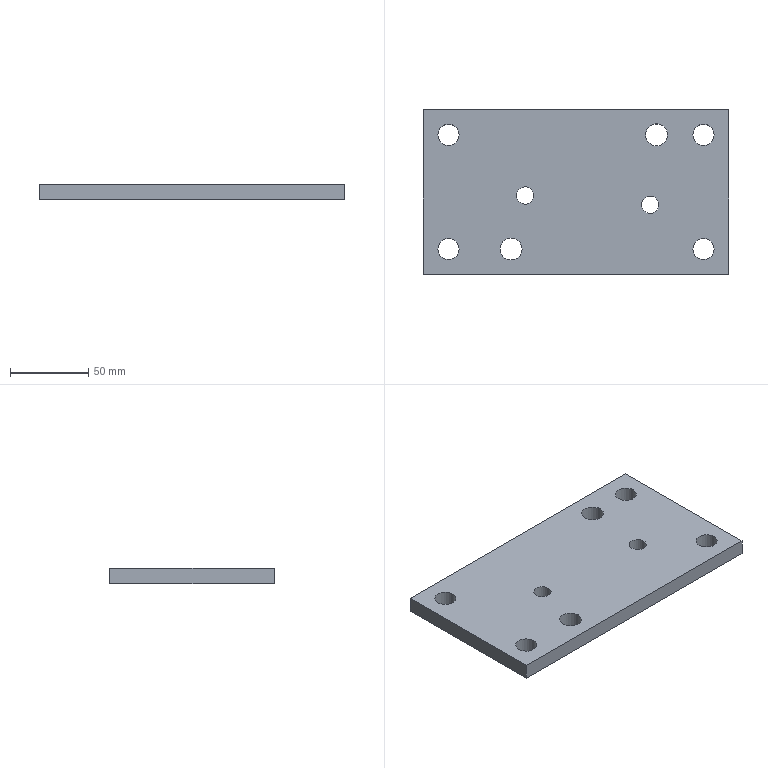Part | STEP file | lll_id2970_x_t | 1 solid | 14 faces | box 195 x 105 x 10 mm | volume 194037 mm3 | cylinder 8 | plane 6 | commonest cylinder face diameters 13.509 x4 11 x2 14 x2
STEP:
#1=CARTESIAN_POINT('',(1360.5,27.75,102.5));
#2=VERTEX_POINT('',#1);
#3=CARTESIAN_POINT('',(1366.,27.75,102.5));
#4=DIRECTION('',(0.,0.,-1.));
#5=DIRECTION('',(-1.,0.,0.));
#6=AXIS2_PLACEMENT_3D('',#3,#4,#5);
#7=CIRCLE('',#6,5.5);
#8=EDGE_CURVE('',#2,#2,#7,.T.);
#9=ORIENTED_EDGE('',*,*,#8,.F.);
#10=EDGE_LOOP('',(#9));
#11=FACE_BOUND('',#10,.T.);
#12=CARTESIAN_POINT('',(1360.5,27.75,92.5));
#13=VERTEX_POINT('',#12);
#14=CARTESIAN_POINT('',(1366.,27.75,92.5));
#15=DIRECTION('',(0.,0.,1.));
#16=DIRECTION('',(-1.,0.,0.));
#17=AXIS2_PLACEMENT_3D('',#14,#15,#16);
#18=CIRCLE('',#17,5.5);
#19=EDGE_CURVE('',#13,#13,#18,.T.);
#20=ORIENTED_EDGE('',*,*,#19,.F.);
#21=EDGE_LOOP('',(#20));
#22=FACE_BOUND('',#21,.T.);
#23=CARTESIAN_POINT('',(1366.,27.75,217.5));
#24=DIRECTION('',(0.,0.,-1.));
#25=DIRECTION('',(-1.,0.,0.));
#26=AXIS2_PLACEMENT_3D('',#23,#24,#25);
#27=CYLINDRICAL_SURFACE('',#26,5.5);
#28=ADVANCED_FACE('',(#11,#22),#27,.F.);
#29=CARTESIAN_POINT('',(1443.,66.5,102.5));
#30=VERTEX_POINT('',#29);
#31=CARTESIAN_POINT('',(1450.,66.5,102.5));
#32=DIRECTION('',(0.,0.,1.));
#33=DIRECTION('',(-1.,0.,0.));
#34=AXIS2_PLACEMENT_3D('',#31,#32,#33);
#35=CIRCLE('',#34,7.);
#36=EDGE_CURVE('',#30,#30,#35,.T.);
#37=ORIENTED_EDGE('',*,*,#36,.T.);
#38=EDGE_LOOP('',(#37));
#39=FACE_BOUND('',#38,.T.);
#40=CARTESIAN_POINT('',(1443.,66.5,92.5));
#41=VERTEX_POINT('',#40);
#42=CARTESIAN_POINT('',(1450.,66.5,92.5));
#43=DIRECTION('',(0.,0.,1.));
#44=DIRECTION('',(-1.,0.,0.));
#45=AXIS2_PLACEMENT_3D('',#42,#43,#44);
#46=CIRCLE('',#45,7.);
#47=EDGE_CURVE('',#41,#41,#46,.T.);
#48=ORIENTED_EDGE('',*,*,#47,.F.);
#49=EDGE_LOOP('',(#48));
#50=FACE_BOUND('',#49,.T.);
#51=CARTESIAN_POINT('',(1450.,66.5,92.5));
#52=DIRECTION('',(0.,0.,1.));
#53=DIRECTION('',(-1.,0.,0.));
#54=AXIS2_PLACEMENT_3D('',#51,#52,#53);
#55=CYLINDRICAL_SURFACE('',#54,7.);
#56=ADVANCED_FACE('',(#39,#50),#55,.F.);
#57=CARTESIAN_POINT('',(1310.245,66.5,102.5));
#58=VERTEX_POINT('',#57);
#59=CARTESIAN_POINT('',(1317.,66.5,102.5));
#60=DIRECTION('',(0.,0.,-1.));
#61=DIRECTION('',(-1.,0.,0.));
#62=AXIS2_PLACEMENT_3D('',#59,#60,#61);
#63=CIRCLE('',#62,6.755);
#64=EDGE_CURVE('',#58,#58,#63,.T.);
#65=ORIENTED_EDGE('',*,*,#64,.F.);
#66=EDGE_LOOP('',(#65));
#67=FACE_BOUND('',#66,.T.);
#68=CARTESIAN_POINT('',(1310.245,66.5,92.5));
#69=VERTEX_POINT('',#68);
#70=CARTESIAN_POINT('',(1317.,66.5,92.5));
#71=DIRECTION('',(0.,0.,1.));
#72=DIRECTION('',(-1.,0.,0.));
#73=AXIS2_PLACEMENT_3D('',#70,#71,#72);
#74=CIRCLE('',#73,6.755);
#75=EDGE_CURVE('',#69,#69,#74,.T.);
#76=ORIENTED_EDGE('',*,*,#75,.F.);
#77=EDGE_LOOP('',(#76));
#78=FACE_BOUND('',#77,.T.);
#79=CARTESIAN_POINT('',(1317.,66.5,92.5));
#80=DIRECTION('',(0.,0.,1.));
#81=DIRECTION('',(-1.,0.,0.));
#82=AXIS2_PLACEMENT_3D('',#79,#80,#81);
#83=CYLINDRICAL_SURFACE('',#82,6.755);
#84=ADVANCED_FACE('',(#67,#78),#83,.F.);
#85=CARTESIAN_POINT('',(1473.245,66.5,102.5));
#86=VERTEX_POINT('',#85);
#87=CARTESIAN_POINT('',(1480.,66.5,102.5));
#88=DIRECTION('',(0.,0.,-1.));
#89=DIRECTION('',(-1.,0.,0.));
#90=AXIS2_PLACEMENT_3D('',#87,#88,#89);
#91=CIRCLE('',#90,6.755);
#92=EDGE_CURVE('',#86,#86,#91,.T.);
#93=ORIENTED_EDGE('',*,*,#92,.F.);
#94=EDGE_LOOP('',(#93));
#95=FACE_BOUND('',#94,.T.);
#96=CARTESIAN_POINT('',(1473.245,66.5,92.5));
#97=VERTEX_POINT('',#96);
#98=CARTESIAN_POINT('',(1480.,66.5,92.5));
#99=DIRECTION('',(0.,0.,1.));
#100=DIRECTION('',(-1.,0.,0.));
#101=AXIS2_PLACEMENT_3D('',#98,#99,#100);
#102=CIRCLE('',#101,6.755);
#103=EDGE_CURVE('',#97,#97,#102,.T.);
#104=ORIENTED_EDGE('',*,*,#103,.F.);
#105=EDGE_LOOP('',(#104));
#106=FACE_BOUND('',#105,.T.);
#107=CARTESIAN_POINT('',(1480.,66.5,92.5));
#108=DIRECTION('',(0.,0.,1.));
#109=DIRECTION('',(-1.,0.,0.));
#110=AXIS2_PLACEMENT_3D('',#107,#108,#109);
#111=CYLINDRICAL_SURFACE('',#110,6.755);
#112=ADVANCED_FACE('',(#95,#106),#111,.F.);
#113=CARTESIAN_POINT('',(1301.,82.5,102.5));
#114=VERTEX_POINT('',#113);
#115=CARTESIAN_POINT('',(1301.,-22.5,102.5));
#116=VERTEX_POINT('',#115);
#117=CARTESIAN_POINT('',(1301.,30.,102.5));
#118=DIRECTION('',(0.,-1.,0.));
#119=VECTOR('',#118,1.);
#120=LINE('',#117,#119);
#121=EDGE_CURVE('',#114,#116,#120,.T.);
#122=ORIENTED_EDGE('',*,*,#121,.F.);
#123=CARTESIAN_POINT('',(1301.,82.5,92.5));
#124=VERTEX_POINT('',#123);
#125=CARTESIAN_POINT('',(1301.,82.5,92.5));
#126=DIRECTION('',(0.,0.,1.));
#127=VECTOR('',#126,1.);
#128=LINE('',#125,#127);
#129=EDGE_CURVE('',#124,#114,#128,.T.);
#130=ORIENTED_EDGE('',*,*,#129,.F.);
#131=CARTESIAN_POINT('',(1301.,-22.5,92.5));
#132=VERTEX_POINT('',#131);
#133=CARTESIAN_POINT('',(1301.,30.,92.5));
#134=DIRECTION('',(0.,-1.,0.));
#135=VECTOR('',#134,1.);
#136=LINE('',#133,#135);
#137=EDGE_CURVE('',#124,#132,#136,.T.);
#138=ORIENTED_EDGE('',*,*,#137,.T.);
#139=CARTESIAN_POINT('',(1301.,-22.5,92.5));
#140=DIRECTION('',(0.,0.,1.));
#141=VECTOR('',#140,1.);
#142=LINE('',#139,#141);
#143=EDGE_CURVE('',#132,#116,#142,.T.);
#144=ORIENTED_EDGE('',*,*,#143,.T.);
#145=EDGE_LOOP('',(#122,#130,#138,#144));
#146=FACE_OUTER_BOUND('',#145,.T.);
#147=CARTESIAN_POINT('',(1301.,30.,92.5));
#148=DIRECTION('',(-1.,0.,0.));
#149=DIRECTION('',(0.,0.,-1.));
#150=AXIS2_PLACEMENT_3D('',#147,#148,#149);
#151=PLANE('',#150);
#152=ADVANCED_FACE('',(#146),#151,.T.);
#153=CARTESIAN_POINT('',(1496.,-22.5,102.5));
#154=VERTEX_POINT('',#153);
#155=CARTESIAN_POINT('',(1398.5,-22.5,102.5));
#156=DIRECTION('',(-1.,0.,0.));
#157=VECTOR('',#156,1.);
#158=LINE('',#155,#157);
#159=EDGE_CURVE('',#154,#116,#158,.T.);
#160=ORIENTED_EDGE('',*,*,#159,.T.);
#161=ORIENTED_EDGE('',*,*,#143,.F.);
#162=CARTESIAN_POINT('',(1496.,-22.5,92.5));
#163=VERTEX_POINT('',#162);
#164=CARTESIAN_POINT('',(1398.5,-22.5,92.5));
#165=DIRECTION('',(1.,0.,0.));
#166=VECTOR('',#165,1.);
#167=LINE('',#164,#166);
#168=EDGE_CURVE('',#132,#163,#167,.T.);
#169=ORIENTED_EDGE('',*,*,#168,.T.);
#170=CARTESIAN_POINT('',(1496.,-22.5,92.5));
#171=DIRECTION('',(0.,0.,1.));
#172=VECTOR('',#171,1.);
#173=LINE('',#170,#172);
#174=EDGE_CURVE('',#163,#154,#173,.T.);
#175=ORIENTED_EDGE('',*,*,#174,.T.);
#176=EDGE_LOOP('',(#160,#161,#169,#175));
#177=FACE_OUTER_BOUND('',#176,.T.);
#178=CARTESIAN_POINT('',(1398.5,-22.5,92.5));
#179=DIRECTION('',(0.,-1.,0.));
#180=DIRECTION('',(0.,0.,1.));
#181=AXIS2_PLACEMENT_3D('',#178,#179,#180);
#182=PLANE('',#181);
#183=ADVANCED_FACE('',(#177),#182,.T.);
#184=CARTESIAN_POINT('',(1496.,82.5,102.5));
#185=VERTEX_POINT('',#184);
#186=CARTESIAN_POINT('',(1496.,30.,102.5));
#187=DIRECTION('',(0.,1.,0.));
#188=VECTOR('',#187,1.);
#189=LINE('',#186,#188);
#190=EDGE_CURVE('',#154,#185,#189,.T.);
#191=ORIENTED_EDGE('',*,*,#190,.F.);
#192=ORIENTED_EDGE('',*,*,#174,.F.);
#193=CARTESIAN_POINT('',(1496.,82.5,92.5));
#194=VERTEX_POINT('',#193);
#195=CARTESIAN_POINT('',(1496.,30.,92.5));
#196=DIRECTION('',(0.,1.,0.));
#197=VECTOR('',#196,1.);
#198=LINE('',#195,#197);
#199=EDGE_CURVE('',#163,#194,#198,.T.);
#200=ORIENTED_EDGE('',*,*,#199,.T.);
#201=CARTESIAN_POINT('',(1496.,82.5,92.5));
#202=DIRECTION('',(0.,0.,1.));
#203=VECTOR('',#202,1.);
#204=LINE('',#201,#203);
#205=EDGE_CURVE('',#194,#185,#204,.T.);
#206=ORIENTED_EDGE('',*,*,#205,.T.);
#207=EDGE_LOOP('',(#191,#192,#200,#206));
#208=FACE_OUTER_BOUND('',#207,.T.);
#209=CARTESIAN_POINT('',(1496.,30.,92.5));
#210=DIRECTION('',(1.,0.,0.));
#211=DIRECTION('',(0.,0.,1.));
#212=AXIS2_PLACEMENT_3D('',#209,#210,#211);
#213=PLANE('',#212);
#214=ADVANCED_FACE('',(#208),#213,.T.);
#215=CARTESIAN_POINT('',(1398.5,82.5,102.5));
#216=DIRECTION('',(1.,0.,0.));
#217=VECTOR('',#216,1.);
#218=LINE('',#215,#217);
#219=EDGE_CURVE('',#114,#185,#218,.T.);
#220=ORIENTED_EDGE('',*,*,#219,.T.);
#221=ORIENTED_EDGE('',*,*,#205,.F.);
#222=CARTESIAN_POINT('',(1398.5,82.5,92.5));
#223=DIRECTION('',(-1.,0.,0.));
#224=VECTOR('',#223,1.);
#225=LINE('',#222,#224);
#226=EDGE_CURVE('',#194,#124,#225,.T.);
#227=ORIENTED_EDGE('',*,*,#226,.T.);
#228=ORIENTED_EDGE('',*,*,#129,.T.);
#229=EDGE_LOOP('',(#220,#221,#227,#228));
#230=FACE_OUTER_BOUND('',#229,.T.);
#231=CARTESIAN_POINT('',(1398.5,82.5,92.5));
#232=DIRECTION('',(0.,1.,0.));
#233=DIRECTION('',(0.,0.,-1.));
#234=AXIS2_PLACEMENT_3D('',#231,#232,#233);
#235=PLANE('',#234);
#236=ADVANCED_FACE('',(#230),#235,.T.);
#237=CARTESIAN_POINT('',(1310.245,-6.5,102.5));
#238=VERTEX_POINT('',#237);
#239=CARTESIAN_POINT('',(1317.,-6.5,102.5));
#240=DIRECTION('',(0.,0.,-1.));
#241=DIRECTION('',(-1.,0.,0.));
#242=AXIS2_PLACEMENT_3D('',#239,#240,#241);
#243=CIRCLE('',#242,6.755);
#244=EDGE_CURVE('',#238,#238,#243,.T.);
#245=ORIENTED_EDGE('',*,*,#244,.F.);
#246=EDGE_LOOP('',(#245));
#247=FACE_BOUND('',#246,.T.);
#248=CARTESIAN_POINT('',(1310.245,-6.5,92.5));
#249=VERTEX_POINT('',#248);
#250=CARTESIAN_POINT('',(1317.,-6.5,92.5));
#251=DIRECTION('',(0.,0.,1.));
#252=DIRECTION('',(-1.,0.,0.));
#253=AXIS2_PLACEMENT_3D('',#250,#251,#252);
#254=CIRCLE('',#253,6.755);
#255=EDGE_CURVE('',#249,#249,#254,.T.);
#256=ORIENTED_EDGE('',*,*,#255,.F.);
#257=EDGE_LOOP('',(#256));
#258=FACE_BOUND('',#257,.T.);
#259=CARTESIAN_POINT('',(1317.,-6.5,92.5));
#260=DIRECTION('',(0.,0.,1.));
#261=DIRECTION('',(-1.,0.,0.));
#262=AXIS2_PLACEMENT_3D('',#259,#260,#261);
#263=CYLINDRICAL_SURFACE('',#262,6.755);
#264=ADVANCED_FACE('',(#247,#258),#263,.F.);
#265=CARTESIAN_POINT('',(1473.245,-6.5,102.5));
#266=VERTEX_POINT('',#265);
#267=CARTESIAN_POINT('',(1480.,-6.5,102.5));
#268=DIRECTION('',(0.,0.,1.));
#269=DIRECTION('',(-1.,0.,0.));
#270=AXIS2_PLACEMENT_3D('',#267,#268,#269);
#271=CIRCLE('',#270,6.755);
#272=EDGE_CURVE('',#266,#266,#271,.T.);
#273=ORIENTED_EDGE('',*,*,#272,.T.);
#274=EDGE_LOOP('',(#273));
#275=FACE_BOUND('',#274,.T.);
#276=CARTESIAN_POINT('',(1473.245,-6.5,92.5));
#277=VERTEX_POINT('',#276);
#278=CARTESIAN_POINT('',(1480.,-6.5,92.5));
#279=DIRECTION('',(0.,0.,1.));
#280=DIRECTION('',(-1.,0.,0.));
#281=AXIS2_PLACEMENT_3D('',#278,#279,#280);
#282=CIRCLE('',#281,6.755);
#283=EDGE_CURVE('',#277,#277,#282,.T.);
#284=ORIENTED_EDGE('',*,*,#283,.F.);
#285=EDGE_LOOP('',(#284));
#286=FACE_BOUND('',#285,.T.);
#287=CARTESIAN_POINT('',(1480.,-6.5,92.5));
#288=DIRECTION('',(0.,0.,1.));
#289=DIRECTION('',(-1.,0.,0.));
#290=AXIS2_PLACEMENT_3D('',#287,#288,#289);
#291=CYLINDRICAL_SURFACE('',#290,6.755);
#292=ADVANCED_FACE('',(#275,#286),#291,.F.);
#293=CARTESIAN_POINT('',(1350.,-6.5,102.5));
#294=VERTEX_POINT('',#293);
#295=CARTESIAN_POINT('',(1357.,-6.5,102.5));
#296=DIRECTION('',(0.,0.,1.));
#297=DIRECTION('',(-1.,0.,0.));
#298=AXIS2_PLACEMENT_3D('',#295,#296,#297);
#299=CIRCLE('',#298,7.);
#300=EDGE_CURVE('',#294,#294,#299,.T.);
#301=ORIENTED_EDGE('',*,*,#300,.T.);
#302=EDGE_LOOP('',(#301));
#303=FACE_BOUND('',#302,.T.);
#304=CARTESIAN_POINT('',(1350.,-6.5,92.5));
#305=VERTEX_POINT('',#304);
#306=CARTESIAN_POINT('',(1357.,-6.5,92.5));
#307=DIRECTION('',(0.,0.,1.));
#308=DIRECTION('',(-1.,0.,0.));
#309=AXIS2_PLACEMENT_3D('',#306,#307,#308);
#310=CIRCLE('',#309,7.);
#311=EDGE_CURVE('',#305,#305,#310,.T.);
#312=ORIENTED_EDGE('',*,*,#311,.F.);
#313=EDGE_LOOP('',(#312));
#314=FACE_BOUND('',#313,.T.);
#315=CARTESIAN_POINT('',(1357.,-6.5,92.5));
#316=DIRECTION('',(0.,0.,1.));
#317=DIRECTION('',(-1.,0.,0.));
#318=AXIS2_PLACEMENT_3D('',#315,#316,#317);
#319=CYLINDRICAL_SURFACE('',#318,7.);
#320=ADVANCED_FACE('',(#303,#314),#319,.F.);
#321=CARTESIAN_POINT('',(1440.5,21.75,92.5));
#322=VERTEX_POINT('',#321);
#323=CARTESIAN_POINT('',(1446.,21.75,92.5));
#324=DIRECTION('',(0.,0.,-1.));
#325=DIRECTION('',(-1.,0.,0.));
#326=AXIS2_PLACEMENT_3D('',#323,#324,#325);
#327=CIRCLE('',#326,5.5);
#328=EDGE_CURVE('',#322,#322,#327,.T.);
#329=ORIENTED_EDGE('',*,*,#328,.F.);
#330=EDGE_LOOP('',(#329));
#331=FACE_BOUND('',#330,.T.);
#332=ORIENTED_EDGE('',*,*,#311,.T.);
#333=EDGE_LOOP('',(#332));
#334=FACE_BOUND('',#333,.T.);
#335=ORIENTED_EDGE('',*,*,#283,.T.);
#336=EDGE_LOOP('',(#335));
#337=FACE_BOUND('',#336,.T.);
#338=ORIENTED_EDGE('',*,*,#255,.T.);
#339=EDGE_LOOP('',(#338));
#340=FACE_BOUND('',#339,.T.);
#341=ORIENTED_EDGE('',*,*,#137,.F.);
#342=ORIENTED_EDGE('',*,*,#226,.F.);
#343=ORIENTED_EDGE('',*,*,#199,.F.);
#344=ORIENTED_EDGE('',*,*,#168,.F.);
#345=EDGE_LOOP('',(#341,#342,#343,#344));
#346=FACE_BOUND('',#345,.T.);
#347=ORIENTED_EDGE('',*,*,#103,.T.);
#348=EDGE_LOOP('',(#347));
#349=FACE_BOUND('',#348,.T.);
#350=ORIENTED_EDGE('',*,*,#75,.T.);
#351=EDGE_LOOP('',(#350));
#352=FACE_BOUND('',#351,.T.);
#353=ORIENTED_EDGE('',*,*,#47,.T.);
#354=EDGE_LOOP('',(#353));
#355=FACE_BOUND('',#354,.T.);
#356=ORIENTED_EDGE('',*,*,#19,.T.);
#357=EDGE_LOOP('',(#356));
#358=FACE_BOUND('',#357,.T.);
#359=CARTESIAN_POINT('',(1398.5,30.,92.5));
#360=DIRECTION('',(0.,0.,-1.));
#361=DIRECTION('',(1.,0.,0.));
#362=AXIS2_PLACEMENT_3D('',#359,#360,#361);
#363=PLANE('',#362);
#364=ADVANCED_FACE('',(#331,#334,#337,#340,#346,#349,#352,#355,#358),#363,.T.);
#365=CARTESIAN_POINT('',(1440.5,21.75,102.5));
#366=VERTEX_POINT('',#365);
#367=CARTESIAN_POINT('',(1446.,21.75,102.5));
#368=DIRECTION('',(0.,0.,1.));
#369=DIRECTION('',(-1.,0.,0.));
#370=AXIS2_PLACEMENT_3D('',#367,#368,#369);
#371=CIRCLE('',#370,5.5);
#372=EDGE_CURVE('',#366,#366,#371,.T.);
#373=ORIENTED_EDGE('',*,*,#372,.T.);
#374=EDGE_LOOP('',(#373));
#375=FACE_BOUND('',#374,.T.);
#376=ORIENTED_EDGE('',*,*,#328,.T.);
#377=EDGE_LOOP('',(#376));
#378=FACE_BOUND('',#377,.T.);
#379=CARTESIAN_POINT('',(1446.,21.75,217.5));
#380=DIRECTION('',(0.,0.,-1.));
#381=DIRECTION('',(-1.,0.,0.));
#382=AXIS2_PLACEMENT_3D('',#379,#380,#381);
#383=CYLINDRICAL_SURFACE('',#382,5.5);
#384=ADVANCED_FACE('',(#375,#378),#383,.F.);
#385=ORIENTED_EDGE('',*,*,#219,.F.);
#386=ORIENTED_EDGE('',*,*,#121,.T.);
#387=ORIENTED_EDGE('',*,*,#159,.F.);
#388=ORIENTED_EDGE('',*,*,#190,.T.);
#389=EDGE_LOOP('',(#385,#386,#387,#388));
#390=FACE_BOUND('',#389,.T.);
#391=ORIENTED_EDGE('',*,*,#244,.T.);
#392=EDGE_LOOP('',(#391));
#393=FACE_BOUND('',#392,.T.);
#394=ORIENTED_EDGE('',*,*,#272,.F.);
#395=EDGE_LOOP('',(#394));
#396=FACE_BOUND('',#395,.T.);
#397=ORIENTED_EDGE('',*,*,#300,.F.);
#398=EDGE_LOOP('',(#397));
#399=FACE_BOUND('',#398,.T.);
#400=ORIENTED_EDGE('',*,*,#8,.T.);
#401=EDGE_LOOP('',(#400));
#402=FACE_BOUND('',#401,.T.);
#403=ORIENTED_EDGE('',*,*,#372,.F.);
#404=EDGE_LOOP('',(#403));
#405=FACE_BOUND('',#404,.T.);
#406=ORIENTED_EDGE('',*,*,#36,.F.);
#407=EDGE_LOOP('',(#406));
#408=FACE_BOUND('',#407,.T.);
#409=ORIENTED_EDGE('',*,*,#64,.T.);
#410=EDGE_LOOP('',(#409));
#411=FACE_BOUND('',#410,.T.);
#412=ORIENTED_EDGE('',*,*,#92,.T.);
#413=EDGE_LOOP('',(#412));
#414=FACE_BOUND('',#413,.T.);
#415=CARTESIAN_POINT('',(1353.5,0.,102.5));
#416=DIRECTION('',(0.,0.,-1.));
#417=DIRECTION('',(-1.,0.,0.));
#418=AXIS2_PLACEMENT_3D('',#415,#416,#417);
#419=PLANE('',#418);
#420=ADVANCED_FACE('',(#390,#393,#396,#399,#402,#405,#408,#411,#414),#419,.F.);
#421=CLOSED_SHELL('',(#28,#56,#84,#112,#152,#183,#214,#236,#264,#292,#320,#364,#384,#420));
#422=MANIFOLD_SOLID_BREP('',#421);
#423=(LENGTH_UNIT()NAMED_UNIT(*)SI_UNIT(.MILLI.,.METRE.));
#424=UNCERTAINTY_MEASURE_WITH_UNIT(LENGTH_MEASURE(0.00002),#423,'','');
#425=(NAMED_UNIT(*)PLANE_ANGLE_UNIT()SI_UNIT($,.RADIAN.));
#426=PLANE_ANGLE_MEASURE_WITH_UNIT(PLANE_ANGLE_MEASURE(0.01745),#425);
#427=DIMENSIONAL_EXPONENTS(0.,0.,0.,0.,0.,0.,0.);
#428=(CONVERSION_BASED_UNIT('DEGREE',#426)NAMED_UNIT(#427)PLANE_ANGLE_UNIT());
#429=(NAMED_UNIT(*)SI_UNIT($,.STERADIAN.)SOLID_ANGLE_UNIT());
#430=(GEOMETRIC_REPRESENTATION_CONTEXT(3)GLOBAL_UNCERTAINTY_ASSIGNED_CONTEXT((#424))GLOBAL_UNIT_ASSIGNED_CONTEXT((#423,#428,#429))REPRESENTATION_CONTEXT('',''));
#431=ADVANCED_BREP_SHAPE_REPRESENTATION('',(#422),#430);